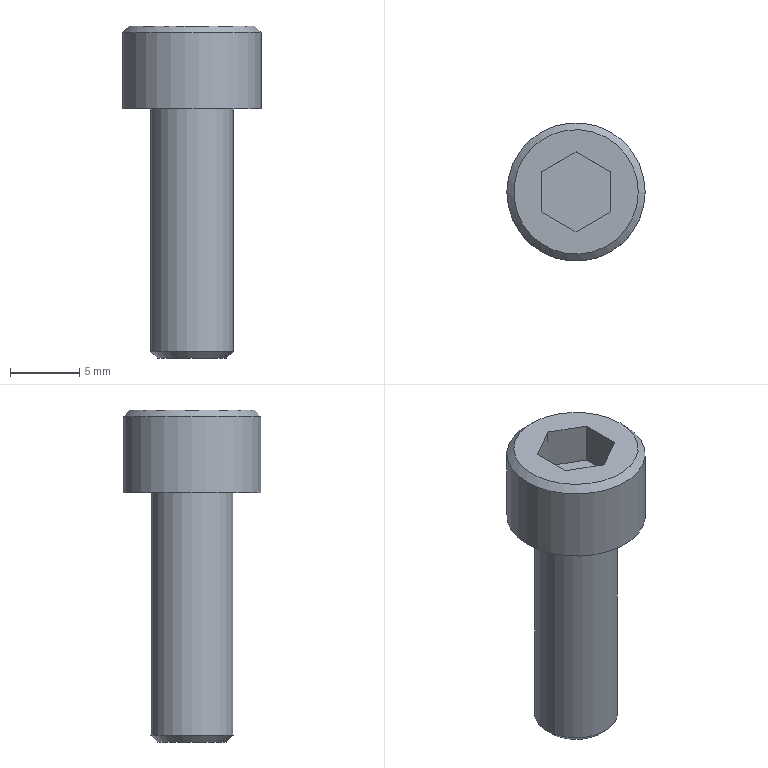Part | NX | features M6.00-20.00 2 | 1 solid | 14 faces | box 10 x 10 x 24 mm | volume 909.204 mm3 | plane 10 | cylinder 2 | cone 2 | commonest cylinder face diameters 6 x1 10 x1
STEP:
#1=CARTESIAN_POINT('',(4.5,100.,-181.5));
#2=VERTEX_POINT('',#1);
#3=CARTESIAN_POINT('',(0.,100.,-181.5));
#4=DIRECTION('',(0.,0.,1.));
#5=DIRECTION('',(1.,0.,0.));
#6=AXIS2_PLACEMENT_3D('',#3,#4,#5);
#7=CIRCLE('',#6,4.5);
#8=EDGE_CURVE('',#2,#2,#7,.T.);
#9=ORIENTED_EDGE('',*,*,#8,.T.);
#10=EDGE_LOOP('',(#9));
#11=FACE_BOUND('',#10,.T.);
#12=CARTESIAN_POINT('',(-2.5,101.443,-181.5));
#13=VERTEX_POINT('',#12);
#14=CARTESIAN_POINT('',(-2.5,98.557,-181.5));
#15=VERTEX_POINT('',#14);
#16=CARTESIAN_POINT('',(-2.5,101.443,-181.5));
#17=DIRECTION('',(0.,-1.,0.));
#18=VECTOR('',#17,1000.);
#19=LINE('',#16,#18);
#20=EDGE_CURVE('',#13,#15,#19,.T.);
#21=ORIENTED_EDGE('',*,*,#20,.F.);
#22=CARTESIAN_POINT('',(0.,102.887,-181.5));
#23=VERTEX_POINT('',#22);
#24=CARTESIAN_POINT('',(0.,102.887,-181.5));
#25=DIRECTION('',(-0.866,-0.5,0.));
#26=VECTOR('',#25,1000.);
#27=LINE('',#24,#26);
#28=EDGE_CURVE('',#23,#13,#27,.T.);
#29=ORIENTED_EDGE('',*,*,#28,.F.);
#30=CARTESIAN_POINT('',(2.5,101.443,-181.5));
#31=VERTEX_POINT('',#30);
#32=CARTESIAN_POINT('',(2.5,101.443,-181.5));
#33=DIRECTION('',(-0.866,0.5,0.));
#34=VECTOR('',#33,1000.);
#35=LINE('',#32,#34);
#36=EDGE_CURVE('',#31,#23,#35,.T.);
#37=ORIENTED_EDGE('',*,*,#36,.F.);
#38=CARTESIAN_POINT('',(2.5,98.557,-181.5));
#39=VERTEX_POINT('',#38);
#40=CARTESIAN_POINT('',(2.5,98.557,-181.5));
#41=DIRECTION('',(0.,1.,0.));
#42=VECTOR('',#41,1000.);
#43=LINE('',#40,#42);
#44=EDGE_CURVE('',#39,#31,#43,.T.);
#45=ORIENTED_EDGE('',*,*,#44,.F.);
#46=CARTESIAN_POINT('',(0.,97.113,-181.5));
#47=VERTEX_POINT('',#46);
#48=CARTESIAN_POINT('',(0.,97.113,-181.5));
#49=DIRECTION('',(0.866,0.5,0.));
#50=VECTOR('',#49,1000.);
#51=LINE('',#48,#50);
#52=EDGE_CURVE('',#47,#39,#51,.T.);
#53=ORIENTED_EDGE('',*,*,#52,.F.);
#54=CARTESIAN_POINT('',(-2.5,98.557,-181.5));
#55=DIRECTION('',(0.866,-0.5,0.));
#56=VECTOR('',#55,1000.);
#57=LINE('',#54,#56);
#58=EDGE_CURVE('',#15,#47,#57,.T.);
#59=ORIENTED_EDGE('',*,*,#58,.F.);
#60=EDGE_LOOP('',(#21,#29,#37,#45,#53,#59));
#61=FACE_BOUND('',#60,.T.);
#62=CARTESIAN_POINT('',(0.,100.,-181.5));
#63=DIRECTION('',(0.,0.,1.));
#64=DIRECTION('',(1.,0.,0.));
#65=AXIS2_PLACEMENT_3D('',#62,#63,#64);
#66=PLANE('',#65);
#67=ADVANCED_FACE('',(#11,#61),#66,.T.);
#68=CARTESIAN_POINT('',(3.,100.,-187.5));
#69=VERTEX_POINT('',#68);
#70=CARTESIAN_POINT('',(0.,100.,-187.5));
#71=DIRECTION('',(0.,0.,-1.));
#72=DIRECTION('',(1.,0.,0.));
#73=AXIS2_PLACEMENT_3D('',#70,#71,#72);
#74=CIRCLE('',#73,3.);
#75=EDGE_CURVE('',#69,#69,#74,.T.);
#76=ORIENTED_EDGE('',*,*,#75,.F.);
#77=EDGE_LOOP('',(#76));
#78=FACE_BOUND('',#77,.T.);
#79=CARTESIAN_POINT('',(5.,100.,-187.5));
#80=VERTEX_POINT('',#79);
#81=CARTESIAN_POINT('',(0.,100.,-187.5));
#82=DIRECTION('',(0.,0.,1.));
#83=DIRECTION('',(1.,0.,0.));
#84=AXIS2_PLACEMENT_3D('',#81,#82,#83);
#85=CIRCLE('',#84,5.);
#86=EDGE_CURVE('',#80,#80,#85,.T.);
#87=ORIENTED_EDGE('',*,*,#86,.F.);
#88=EDGE_LOOP('',(#87));
#89=FACE_BOUND('',#88,.T.);
#90=CARTESIAN_POINT('',(0.,100.,-187.5));
#91=DIRECTION('',(0.,0.,-1.));
#92=DIRECTION('',(-1.,0.,0.));
#93=AXIS2_PLACEMENT_3D('',#90,#91,#92);
#94=PLANE('',#93);
#95=ADVANCED_FACE('',(#78,#89),#94,.T.);
#96=CARTESIAN_POINT('',(5.,100.,-182.));
#97=VERTEX_POINT('',#96);
#98=CARTESIAN_POINT('',(0.,100.,-182.));
#99=DIRECTION('',(0.,0.,1.));
#100=DIRECTION('',(1.,0.,0.));
#101=AXIS2_PLACEMENT_3D('',#98,#99,#100);
#102=CIRCLE('',#101,5.);
#103=EDGE_CURVE('',#97,#97,#102,.F.);
#104=ORIENTED_EDGE('',*,*,#103,.T.);
#105=EDGE_LOOP('',(#104));
#106=FACE_BOUND('',#105,.T.);
#107=ORIENTED_EDGE('',*,*,#86,.T.);
#108=EDGE_LOOP('',(#107));
#109=FACE_BOUND('',#108,.T.);
#110=CARTESIAN_POINT('',(0.,100.,-187.5));
#111=DIRECTION('',(0.,0.,1.));
#112=DIRECTION('',(1.,0.,0.));
#113=AXIS2_PLACEMENT_3D('',#110,#111,#112);
#114=CYLINDRICAL_SURFACE('',#113,5.);
#115=ADVANCED_FACE('',(#106,#109),#114,.T.);
#116=CARTESIAN_POINT('',(-2.5,100.,-205.5));
#117=VERTEX_POINT('',#116);
#118=CARTESIAN_POINT('',(0.,100.,-205.5));
#119=DIRECTION('',(0.,0.,-1.));
#120=DIRECTION('',(-1.,0.,0.));
#121=AXIS2_PLACEMENT_3D('',#118,#119,#120);
#122=CIRCLE('',#121,2.5);
#123=EDGE_CURVE('',#117,#117,#122,.T.);
#124=ORIENTED_EDGE('',*,*,#123,.T.);
#125=EDGE_LOOP('',(#124));
#126=FACE_BOUND('',#125,.T.);
#127=CARTESIAN_POINT('',(0.,100.,-205.5));
#128=DIRECTION('',(0.,0.,-1.));
#129=DIRECTION('',(-1.,0.,0.));
#130=AXIS2_PLACEMENT_3D('',#127,#128,#129);
#131=PLANE('',#130);
#132=ADVANCED_FACE('',(#126),#131,.T.);
#133=CARTESIAN_POINT('',(-3.,100.,-205.));
#134=VERTEX_POINT('',#133);
#135=CARTESIAN_POINT('',(0.,100.,-205.));
#136=DIRECTION('',(0.,0.,-1.));
#137=DIRECTION('',(-1.,0.,0.));
#138=AXIS2_PLACEMENT_3D('',#135,#136,#137);
#139=CIRCLE('',#138,3.);
#140=EDGE_CURVE('',#134,#134,#139,.F.);
#141=ORIENTED_EDGE('',*,*,#140,.T.);
#142=EDGE_LOOP('',(#141));
#143=FACE_BOUND('',#142,.T.);
#144=ORIENTED_EDGE('',*,*,#75,.T.);
#145=EDGE_LOOP('',(#144));
#146=FACE_BOUND('',#145,.T.);
#147=CARTESIAN_POINT('',(0.,100.,-187.5));
#148=DIRECTION('',(0.,0.,-1.));
#149=DIRECTION('',(1.,0.,0.));
#150=AXIS2_PLACEMENT_3D('',#147,#148,#149);
#151=CYLINDRICAL_SURFACE('',#150,3.);
#152=ADVANCED_FACE('',(#143,#146),#151,.T.);
#153=ORIENTED_EDGE('',*,*,#58,.T.);
#154=CARTESIAN_POINT('',(0.,97.113,-184.5));
#155=VERTEX_POINT('',#154);
#156=CARTESIAN_POINT('',(0.,97.113,-184.5));
#157=DIRECTION('',(0.,0.,1.));
#158=VECTOR('',#157,1000.);
#159=LINE('',#156,#158);
#160=EDGE_CURVE('',#47,#155,#159,.F.);
#161=ORIENTED_EDGE('',*,*,#160,.T.);
#162=CARTESIAN_POINT('',(-2.5,98.557,-184.5));
#163=VERTEX_POINT('',#162);
#164=CARTESIAN_POINT('',(-2.5,98.557,-184.5));
#165=DIRECTION('',(0.866,-0.5,0.));
#166=VECTOR('',#165,1000.);
#167=LINE('',#164,#166);
#168=EDGE_CURVE('',#155,#163,#167,.F.);
#169=ORIENTED_EDGE('',*,*,#168,.T.);
#170=CARTESIAN_POINT('',(-2.5,98.557,-184.5));
#171=DIRECTION('',(0.,0.,1.));
#172=VECTOR('',#171,1000.);
#173=LINE('',#170,#172);
#174=EDGE_CURVE('',#15,#163,#173,.F.);
#175=ORIENTED_EDGE('',*,*,#174,.F.);
#176=EDGE_LOOP('',(#153,#161,#169,#175));
#177=FACE_BOUND('',#176,.T.);
#178=CARTESIAN_POINT('',(-1.25,97.835,-183.));
#179=DIRECTION('',(-0.5,-0.866,0.));
#180=DIRECTION('',(0.866,-0.5,0.));
#181=AXIS2_PLACEMENT_3D('',#178,#179,#180);
#182=PLANE('',#181);
#183=ADVANCED_FACE('',(#177),#182,.F.);
#184=ORIENTED_EDGE('',*,*,#20,.T.);
#185=ORIENTED_EDGE('',*,*,#174,.T.);
#186=CARTESIAN_POINT('',(-2.5,101.443,-184.5));
#187=VERTEX_POINT('',#186);
#188=CARTESIAN_POINT('',(-2.5,101.443,-184.5));
#189=DIRECTION('',(0.,-1.,0.));
#190=VECTOR('',#189,1000.);
#191=LINE('',#188,#190);
#192=EDGE_CURVE('',#163,#187,#191,.F.);
#193=ORIENTED_EDGE('',*,*,#192,.T.);
#194=CARTESIAN_POINT('',(-2.5,101.443,-184.5));
#195=DIRECTION('',(0.,0.,1.));
#196=VECTOR('',#195,1000.);
#197=LINE('',#194,#196);
#198=EDGE_CURVE('',#13,#187,#197,.F.);
#199=ORIENTED_EDGE('',*,*,#198,.F.);
#200=EDGE_LOOP('',(#184,#185,#193,#199));
#201=FACE_BOUND('',#200,.T.);
#202=CARTESIAN_POINT('',(-2.5,100.,-183.));
#203=DIRECTION('',(-1.,0.,0.));
#204=DIRECTION('',(0.,0.,1.));
#205=AXIS2_PLACEMENT_3D('',#202,#203,#204);
#206=PLANE('',#205);
#207=ADVANCED_FACE('',(#201),#206,.F.);
#208=ORIENTED_EDGE('',*,*,#28,.T.);
#209=ORIENTED_EDGE('',*,*,#198,.T.);
#210=CARTESIAN_POINT('',(0.,102.887,-184.5));
#211=VERTEX_POINT('',#210);
#212=CARTESIAN_POINT('',(0.,102.887,-184.5));
#213=DIRECTION('',(-0.866,-0.5,0.));
#214=VECTOR('',#213,1000.);
#215=LINE('',#212,#214);
#216=EDGE_CURVE('',#187,#211,#215,.F.);
#217=ORIENTED_EDGE('',*,*,#216,.T.);
#218=CARTESIAN_POINT('',(0.,102.887,-184.5));
#219=DIRECTION('',(0.,0.,1.));
#220=VECTOR('',#219,1000.);
#221=LINE('',#218,#220);
#222=EDGE_CURVE('',#23,#211,#221,.F.);
#223=ORIENTED_EDGE('',*,*,#222,.F.);
#224=EDGE_LOOP('',(#208,#209,#217,#223));
#225=FACE_BOUND('',#224,.T.);
#226=CARTESIAN_POINT('',(-1.25,102.165,-183.));
#227=DIRECTION('',(-0.5,0.866,0.));
#228=DIRECTION('',(-0.866,-0.5,0.));
#229=AXIS2_PLACEMENT_3D('',#226,#227,#228);
#230=PLANE('',#229);
#231=ADVANCED_FACE('',(#225),#230,.F.);
#232=ORIENTED_EDGE('',*,*,#36,.T.);
#233=ORIENTED_EDGE('',*,*,#222,.T.);
#234=CARTESIAN_POINT('',(2.5,101.443,-184.5));
#235=VERTEX_POINT('',#234);
#236=CARTESIAN_POINT('',(2.5,101.443,-184.5));
#237=DIRECTION('',(-0.866,0.5,0.));
#238=VECTOR('',#237,1000.);
#239=LINE('',#236,#238);
#240=EDGE_CURVE('',#211,#235,#239,.F.);
#241=ORIENTED_EDGE('',*,*,#240,.T.);
#242=CARTESIAN_POINT('',(2.5,101.443,-184.5));
#243=DIRECTION('',(0.,0.,1.));
#244=VECTOR('',#243,1000.);
#245=LINE('',#242,#244);
#246=EDGE_CURVE('',#31,#235,#245,.F.);
#247=ORIENTED_EDGE('',*,*,#246,.F.);
#248=EDGE_LOOP('',(#232,#233,#241,#247));
#249=FACE_BOUND('',#248,.T.);
#250=CARTESIAN_POINT('',(1.25,102.165,-183.));
#251=DIRECTION('',(0.5,0.866,0.));
#252=DIRECTION('',(-0.866,0.5,0.));
#253=AXIS2_PLACEMENT_3D('',#250,#251,#252);
#254=PLANE('',#253);
#255=ADVANCED_FACE('',(#249),#254,.F.);
#256=ORIENTED_EDGE('',*,*,#44,.T.);
#257=ORIENTED_EDGE('',*,*,#246,.T.);
#258=CARTESIAN_POINT('',(2.5,98.557,-184.5));
#259=VERTEX_POINT('',#258);
#260=CARTESIAN_POINT('',(2.5,98.557,-184.5));
#261=DIRECTION('',(0.,1.,0.));
#262=VECTOR('',#261,1000.);
#263=LINE('',#260,#262);
#264=EDGE_CURVE('',#235,#259,#263,.F.);
#265=ORIENTED_EDGE('',*,*,#264,.T.);
#266=CARTESIAN_POINT('',(2.5,98.557,-184.5));
#267=DIRECTION('',(0.,0.,1.));
#268=VECTOR('',#267,1000.);
#269=LINE('',#266,#268);
#270=EDGE_CURVE('',#39,#259,#269,.F.);
#271=ORIENTED_EDGE('',*,*,#270,.F.);
#272=EDGE_LOOP('',(#256,#257,#265,#271));
#273=FACE_BOUND('',#272,.T.);
#274=CARTESIAN_POINT('',(2.5,100.,-183.));
#275=DIRECTION('',(1.,0.,0.));
#276=DIRECTION('',(0.,0.,-1.));
#277=AXIS2_PLACEMENT_3D('',#274,#275,#276);
#278=PLANE('',#277);
#279=ADVANCED_FACE('',(#273),#278,.F.);
#280=ORIENTED_EDGE('',*,*,#52,.T.);
#281=ORIENTED_EDGE('',*,*,#270,.T.);
#282=CARTESIAN_POINT('',(0.,97.113,-184.5));
#283=DIRECTION('',(0.866,0.5,0.));
#284=VECTOR('',#283,1000.);
#285=LINE('',#282,#284);
#286=EDGE_CURVE('',#259,#155,#285,.F.);
#287=ORIENTED_EDGE('',*,*,#286,.T.);
#288=ORIENTED_EDGE('',*,*,#160,.F.);
#289=EDGE_LOOP('',(#280,#281,#287,#288));
#290=FACE_BOUND('',#289,.T.);
#291=CARTESIAN_POINT('',(1.25,97.835,-183.));
#292=DIRECTION('',(0.5,-0.866,0.));
#293=DIRECTION('',(0.866,0.5,0.));
#294=AXIS2_PLACEMENT_3D('',#291,#292,#293);
#295=PLANE('',#294);
#296=ADVANCED_FACE('',(#290),#295,.F.);
#297=ORIENTED_EDGE('',*,*,#286,.F.);
#298=ORIENTED_EDGE('',*,*,#264,.F.);
#299=ORIENTED_EDGE('',*,*,#240,.F.);
#300=ORIENTED_EDGE('',*,*,#216,.F.);
#301=ORIENTED_EDGE('',*,*,#192,.F.);
#302=ORIENTED_EDGE('',*,*,#168,.F.);
#303=EDGE_LOOP('',(#297,#298,#299,#300,#301,#302));
#304=FACE_BOUND('',#303,.T.);
#305=CARTESIAN_POINT('',(0.,100.,-184.5));
#306=DIRECTION('',(0.,0.,-1.));
#307=DIRECTION('',(-1.,0.,0.));
#308=AXIS2_PLACEMENT_3D('',#305,#306,#307);
#309=PLANE('',#308);
#310=ADVANCED_FACE('',(#304),#309,.F.);
#311=ORIENTED_EDGE('',*,*,#123,.F.);
#312=EDGE_LOOP('',(#311));
#313=FACE_BOUND('',#312,.T.);
#314=ORIENTED_EDGE('',*,*,#140,.F.);
#315=EDGE_LOOP('',(#314));
#316=FACE_BOUND('',#315,.T.);
#317=CARTESIAN_POINT('',(0.,100.,-205.));
#318=DIRECTION('',(0.,0.,1.));
#319=DIRECTION('',(1.,0.,0.));
#320=AXIS2_PLACEMENT_3D('',#317,#318,#319);
#321=CONICAL_SURFACE('',#320,3.,0.7854);
#322=ADVANCED_FACE('',(#313,#316),#321,.T.);
#323=ORIENTED_EDGE('',*,*,#8,.F.);
#324=EDGE_LOOP('',(#323));
#325=FACE_BOUND('',#324,.T.);
#326=ORIENTED_EDGE('',*,*,#103,.F.);
#327=EDGE_LOOP('',(#326));
#328=FACE_BOUND('',#327,.T.);
#329=CARTESIAN_POINT('',(0.,100.,-182.));
#330=DIRECTION('',(0.,0.,-1.));
#331=DIRECTION('',(-1.,0.,0.));
#332=AXIS2_PLACEMENT_3D('',#329,#330,#331);
#333=CONICAL_SURFACE('',#332,5.,0.7854);
#334=ADVANCED_FACE('',(#325,#328),#333,.T.);
#335=CLOSED_SHELL('',(#67,#95,#115,#132,#152,#183,#207,#231,#255,#279,#296,#310,#322,#334));
#336=MANIFOLD_SOLID_BREP('',#335);
#337=(LENGTH_UNIT()NAMED_UNIT(*)SI_UNIT(.MILLI.,.METRE.));
#338=UNCERTAINTY_MEASURE_WITH_UNIT(LENGTH_MEASURE(0.00001),#337,'','');
#339=(NAMED_UNIT(*)PLANE_ANGLE_UNIT()SI_UNIT($,.RADIAN.));
#340=(NAMED_UNIT(*)SI_UNIT($,.STERADIAN.)SOLID_ANGLE_UNIT());
#341=(GEOMETRIC_REPRESENTATION_CONTEXT(3)GLOBAL_UNCERTAINTY_ASSIGNED_CONTEXT((#338))GLOBAL_UNIT_ASSIGNED_CONTEXT((#337,#339,#340))REPRESENTATION_CONTEXT('',''));
#342=ADVANCED_BREP_SHAPE_REPRESENTATION('',(#336),#341);